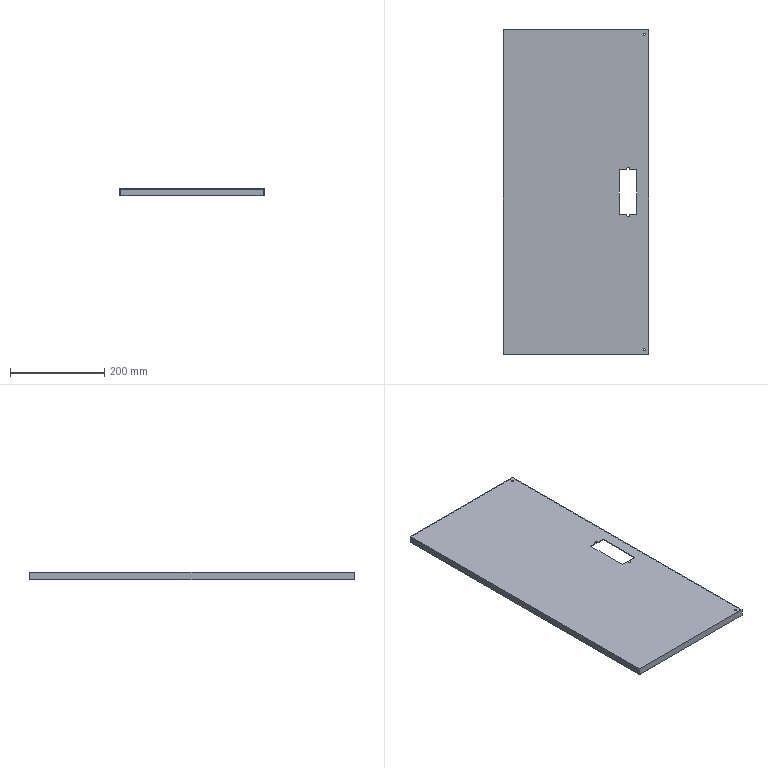Part | SolidWorks | features BaseBody 1 | 1 solid | 27 faces | box 308 x 688 x 15 mm | volume 352674 mm3 | plane 21 | cylinder 6 | commonest cylinder face diameters 4.5 x4 6 x2
STEP:
#1=CARTESIAN_POINT('',(-8.25,334.5,0.));
#2=VERTEX_POINT('',#1);
#3=CARTESIAN_POINT('',(-12.75,334.5,0.));
#4=VERTEX_POINT('',#3);
#5=CARTESIAN_POINT('',(-10.5,334.5,0.));
#6=DIRECTION('',(0.,0.,-1.));
#7=DIRECTION('',(-1.,0.,0.));
#8=AXIS2_PLACEMENT_3D('',#5,#6,#7);
#9=CIRCLE('',#8,2.25);
#10=EDGE_CURVE('',#2,#4,#9,.T.);
#11=ORIENTED_EDGE('',*,*,#10,.F.);
#12=CARTESIAN_POINT('',(-8.25,334.5,-1.5));
#13=VERTEX_POINT('',#12);
#14=CARTESIAN_POINT('',(-8.25,334.5,0.));
#15=DIRECTION('',(0.,0.,-1.));
#16=VECTOR('',#15,1000.);
#17=LINE('',#14,#16);
#18=EDGE_CURVE('',#2,#13,#17,.T.);
#19=ORIENTED_EDGE('',*,*,#18,.T.);
#20=CARTESIAN_POINT('',(-12.75,334.5,-1.5));
#21=VERTEX_POINT('',#20);
#22=CARTESIAN_POINT('',(-10.5,334.5,-1.5));
#23=DIRECTION('',(0.,0.,1.));
#24=DIRECTION('',(-1.,0.,0.));
#25=AXIS2_PLACEMENT_3D('',#22,#23,#24);
#26=CIRCLE('',#25,2.25);
#27=EDGE_CURVE('',#21,#13,#26,.T.);
#28=ORIENTED_EDGE('',*,*,#27,.F.);
#29=CARTESIAN_POINT('',(-12.75,334.5,0.));
#30=DIRECTION('',(0.,0.,-1.));
#31=VECTOR('',#30,1000.);
#32=LINE('',#29,#31);
#33=EDGE_CURVE('',#4,#21,#32,.T.);
#34=ORIENTED_EDGE('',*,*,#33,.F.);
#35=EDGE_LOOP('',(#11,#19,#28,#34));
#36=FACE_OUTER_BOUND('',#35,.T.);
#37=CARTESIAN_POINT('',(-10.5,334.5,0.));
#38=DIRECTION('',(0.,0.,-1.));
#39=DIRECTION('',(-1.,0.,0.));
#40=AXIS2_PLACEMENT_3D('',#37,#38,#39);
#41=CYLINDRICAL_SURFACE('',#40,2.25);
#42=ADVANCED_FACE('',(#36),#41,.F.);
#43=CARTESIAN_POINT('',(-8.25,-334.5,0.));
#44=VERTEX_POINT('',#43);
#45=CARTESIAN_POINT('',(-12.75,-334.5,0.));
#46=VERTEX_POINT('',#45);
#47=CARTESIAN_POINT('',(-10.5,-334.5,0.));
#48=DIRECTION('',(0.,0.,-1.));
#49=DIRECTION('',(-1.,0.,0.));
#50=AXIS2_PLACEMENT_3D('',#47,#48,#49);
#51=CIRCLE('',#50,2.25);
#52=EDGE_CURVE('',#44,#46,#51,.T.);
#53=ORIENTED_EDGE('',*,*,#52,.F.);
#54=CARTESIAN_POINT('',(-8.25,-334.5,-1.5));
#55=VERTEX_POINT('',#54);
#56=CARTESIAN_POINT('',(-8.25,-334.5,0.));
#57=DIRECTION('',(0.,0.,-1.));
#58=VECTOR('',#57,1000.);
#59=LINE('',#56,#58);
#60=EDGE_CURVE('',#44,#55,#59,.T.);
#61=ORIENTED_EDGE('',*,*,#60,.T.);
#62=CARTESIAN_POINT('',(-12.75,-334.5,-1.5));
#63=VERTEX_POINT('',#62);
#64=CARTESIAN_POINT('',(-10.5,-334.5,-1.5));
#65=DIRECTION('',(0.,0.,1.));
#66=DIRECTION('',(-1.,0.,0.));
#67=AXIS2_PLACEMENT_3D('',#64,#65,#66);
#68=CIRCLE('',#67,2.25);
#69=EDGE_CURVE('',#63,#55,#68,.T.);
#70=ORIENTED_EDGE('',*,*,#69,.F.);
#71=CARTESIAN_POINT('',(-12.75,-334.5,0.));
#72=DIRECTION('',(0.,0.,-1.));
#73=VECTOR('',#72,1000.);
#74=LINE('',#71,#73);
#75=EDGE_CURVE('',#46,#63,#74,.T.);
#76=ORIENTED_EDGE('',*,*,#75,.F.);
#77=EDGE_LOOP('',(#53,#61,#70,#76));
#78=FACE_OUTER_BOUND('',#77,.T.);
#79=CARTESIAN_POINT('',(-10.5,-334.5,0.));
#80=DIRECTION('',(0.,0.,-1.));
#81=DIRECTION('',(-1.,0.,0.));
#82=AXIS2_PLACEMENT_3D('',#79,#80,#81);
#83=CYLINDRICAL_SURFACE('',#82,2.25);
#84=ADVANCED_FACE('',(#78),#83,.F.);
#85=CARTESIAN_POINT('',(-1.,-344.,0.));
#86=VERTEX_POINT('',#85);
#87=CARTESIAN_POINT('',(-1.,344.,0.));
#88=VERTEX_POINT('',#87);
#89=CARTESIAN_POINT('',(-1.,0.,0.));
#90=DIRECTION('',(0.,1.,0.));
#91=VECTOR('',#90,1000.);
#92=LINE('',#89,#91);
#93=EDGE_CURVE('',#86,#88,#92,.T.);
#94=ORIENTED_EDGE('',*,*,#93,.T.);
#95=CARTESIAN_POINT('',(-309.,344.,0.));
#96=VERTEX_POINT('',#95);
#97=CARTESIAN_POINT('',(0.,344.,0.));
#98=DIRECTION('',(-1.,0.,0.));
#99=VECTOR('',#98,1000.);
#100=LINE('',#97,#99);
#101=EDGE_CURVE('',#88,#96,#100,.T.);
#102=ORIENTED_EDGE('',*,*,#101,.T.);
#103=CARTESIAN_POINT('',(-309.,-344.,0.));
#104=VERTEX_POINT('',#103);
#105=CARTESIAN_POINT('',(-309.,0.,0.));
#106=DIRECTION('',(0.,-1.,0.));
#107=VECTOR('',#106,1000.);
#108=LINE('',#105,#107);
#109=EDGE_CURVE('',#96,#104,#108,.T.);
#110=ORIENTED_EDGE('',*,*,#109,.T.);
#111=CARTESIAN_POINT('',(0.,-344.,0.));
#112=DIRECTION('',(1.,0.,0.));
#113=VECTOR('',#112,1000.);
#114=LINE('',#111,#113);
#115=EDGE_CURVE('',#104,#86,#114,.T.);
#116=ORIENTED_EDGE('',*,*,#115,.T.);
#117=EDGE_LOOP('',(#94,#102,#110,#116));
#118=FACE_OUTER_BOUND('',#117,.T.);
#119=CARTESIAN_POINT('',(-47.5,-49.5,0.));
#120=VERTEX_POINT('',#119);
#121=CARTESIAN_POINT('',(-47.5,-47.5,0.));
#122=VERTEX_POINT('',#121);
#123=CARTESIAN_POINT('',(-47.5,0.,0.));
#124=DIRECTION('',(0.,1.,0.));
#125=VECTOR('',#124,1000.);
#126=LINE('',#123,#125);
#127=EDGE_CURVE('',#120,#122,#126,.T.);
#128=ORIENTED_EDGE('',*,*,#127,.T.);
#129=CARTESIAN_POINT('',(-63.,-47.5,0.));
#130=VERTEX_POINT('',#129);
#131=CARTESIAN_POINT('',(0.,-47.5,0.));
#132=DIRECTION('',(-1.,0.,0.));
#133=VECTOR('',#132,1000.);
#134=LINE('',#131,#133);
#135=EDGE_CURVE('',#122,#130,#134,.T.);
#136=ORIENTED_EDGE('',*,*,#135,.T.);
#137=CARTESIAN_POINT('',(-63.,47.5,0.));
#138=VERTEX_POINT('',#137);
#139=CARTESIAN_POINT('',(-63.,0.,0.));
#140=DIRECTION('',(0.,1.,0.));
#141=VECTOR('',#140,1000.);
#142=LINE('',#139,#141);
#143=EDGE_CURVE('',#130,#138,#142,.T.);
#144=ORIENTED_EDGE('',*,*,#143,.T.);
#145=CARTESIAN_POINT('',(-47.5,47.5,0.));
#146=VERTEX_POINT('',#145);
#147=CARTESIAN_POINT('',(0.,47.5,0.));
#148=DIRECTION('',(1.,0.,0.));
#149=VECTOR('',#148,1000.);
#150=LINE('',#147,#149);
#151=EDGE_CURVE('',#138,#146,#150,.T.);
#152=ORIENTED_EDGE('',*,*,#151,.T.);
#153=CARTESIAN_POINT('',(-47.5,49.5,0.));
#154=VERTEX_POINT('',#153);
#155=CARTESIAN_POINT('',(-47.5,0.,0.));
#156=DIRECTION('',(0.,1.,0.));
#157=VECTOR('',#156,1000.);
#158=LINE('',#155,#157);
#159=EDGE_CURVE('',#146,#154,#158,.T.);
#160=ORIENTED_EDGE('',*,*,#159,.T.);
#161=CARTESIAN_POINT('',(-41.5,49.5,0.));
#162=VERTEX_POINT('',#161);
#163=CARTESIAN_POINT('',(-44.5,49.5,0.));
#164=DIRECTION('',(0.,0.,-1.));
#165=DIRECTION('',(1.,0.,0.));
#166=AXIS2_PLACEMENT_3D('',#163,#164,#165);
#167=CIRCLE('',#166,3.);
#168=EDGE_CURVE('',#154,#162,#167,.T.);
#169=ORIENTED_EDGE('',*,*,#168,.T.);
#170=CARTESIAN_POINT('',(-41.5,47.5,0.));
#171=VERTEX_POINT('',#170);
#172=CARTESIAN_POINT('',(-41.5,0.,0.));
#173=DIRECTION('',(0.,-1.,0.));
#174=VECTOR('',#173,1000.);
#175=LINE('',#172,#174);
#176=EDGE_CURVE('',#162,#171,#175,.T.);
#177=ORIENTED_EDGE('',*,*,#176,.T.);
#178=CARTESIAN_POINT('',(-26.,47.5,0.));
#179=VERTEX_POINT('',#178);
#180=CARTESIAN_POINT('',(0.,47.5,0.));
#181=DIRECTION('',(1.,0.,0.));
#182=VECTOR('',#181,1000.);
#183=LINE('',#180,#182);
#184=EDGE_CURVE('',#171,#179,#183,.T.);
#185=ORIENTED_EDGE('',*,*,#184,.T.);
#186=CARTESIAN_POINT('',(-26.,-47.5,0.));
#187=VERTEX_POINT('',#186);
#188=CARTESIAN_POINT('',(-26.,0.,0.));
#189=DIRECTION('',(0.,-1.,0.));
#190=VECTOR('',#189,1000.);
#191=LINE('',#188,#190);
#192=EDGE_CURVE('',#179,#187,#191,.T.);
#193=ORIENTED_EDGE('',*,*,#192,.T.);
#194=CARTESIAN_POINT('',(-41.5,-47.5,0.));
#195=VERTEX_POINT('',#194);
#196=CARTESIAN_POINT('',(0.,-47.5,0.));
#197=DIRECTION('',(-1.,0.,0.));
#198=VECTOR('',#197,1000.);
#199=LINE('',#196,#198);
#200=EDGE_CURVE('',#187,#195,#199,.T.);
#201=ORIENTED_EDGE('',*,*,#200,.T.);
#202=CARTESIAN_POINT('',(-41.5,-49.5,0.));
#203=VERTEX_POINT('',#202);
#204=CARTESIAN_POINT('',(-41.5,0.,0.));
#205=DIRECTION('',(0.,-1.,0.));
#206=VECTOR('',#205,1000.);
#207=LINE('',#204,#206);
#208=EDGE_CURVE('',#195,#203,#207,.T.);
#209=ORIENTED_EDGE('',*,*,#208,.T.);
#210=CARTESIAN_POINT('',(-44.5,-49.5,0.));
#211=DIRECTION('',(0.,0.,-1.));
#212=DIRECTION('',(1.,0.,0.));
#213=AXIS2_PLACEMENT_3D('',#210,#211,#212);
#214=CIRCLE('',#213,3.);
#215=EDGE_CURVE('',#203,#120,#214,.T.);
#216=ORIENTED_EDGE('',*,*,#215,.T.);
#217=EDGE_LOOP('',(#128,#136,#144,#152,#160,#169,#177,#185,#193,#201,#209,#216));
#218=FACE_BOUND('',#217,.T.);
#219=CARTESIAN_POINT('',(-10.5,334.5,0.));
#220=DIRECTION('',(0.,0.,-1.));
#221=DIRECTION('',(-1.,0.,0.));
#222=AXIS2_PLACEMENT_3D('',#219,#220,#221);
#223=CIRCLE('',#222,2.25);
#224=EDGE_CURVE('',#4,#2,#223,.T.);
#225=ORIENTED_EDGE('',*,*,#224,.T.);
#226=ORIENTED_EDGE('',*,*,#10,.T.);
#227=EDGE_LOOP('',(#225,#226));
#228=FACE_BOUND('',#227,.T.);
#229=CARTESIAN_POINT('',(-10.5,-334.5,0.));
#230=DIRECTION('',(0.,0.,-1.));
#231=DIRECTION('',(-1.,0.,0.));
#232=AXIS2_PLACEMENT_3D('',#229,#230,#231);
#233=CIRCLE('',#232,2.25);
#234=EDGE_CURVE('',#46,#44,#233,.T.);
#235=ORIENTED_EDGE('',*,*,#234,.T.);
#236=ORIENTED_EDGE('',*,*,#52,.T.);
#237=EDGE_LOOP('',(#235,#236));
#238=FACE_BOUND('',#237,.T.);
#239=CARTESIAN_POINT('',(0.,0.,0.));
#240=DIRECTION('',(0.,0.,1.));
#241=DIRECTION('',(1.,0.,0.));
#242=AXIS2_PLACEMENT_3D('',#239,#240,#241);
#243=PLANE('',#242);
#244=ADVANCED_FACE('',(#118,#218,#228,#238),#243,.T.);
#245=CARTESIAN_POINT('',(-1.,344.,-15.));
#246=VERTEX_POINT('',#245);
#247=CARTESIAN_POINT('',(-309.,344.,-15.));
#248=VERTEX_POINT('',#247);
#249=CARTESIAN_POINT('',(-309.,344.,-15.));
#250=DIRECTION('',(-1.,0.,0.));
#251=VECTOR('',#250,1000.);
#252=LINE('',#249,#251);
#253=EDGE_CURVE('',#246,#248,#252,.T.);
#254=ORIENTED_EDGE('',*,*,#253,.T.);
#255=CARTESIAN_POINT('',(-309.,344.,-15.));
#256=DIRECTION('',(0.,0.,1.));
#257=VECTOR('',#256,1000.);
#258=LINE('',#255,#257);
#259=EDGE_CURVE('',#248,#96,#258,.T.);
#260=ORIENTED_EDGE('',*,*,#259,.T.);
#261=ORIENTED_EDGE('',*,*,#101,.F.);
#262=CARTESIAN_POINT('',(-1.,344.,-15.));
#263=DIRECTION('',(0.,0.,-1.));
#264=VECTOR('',#263,1000.);
#265=LINE('',#262,#264);
#266=EDGE_CURVE('',#88,#246,#265,.T.);
#267=ORIENTED_EDGE('',*,*,#266,.T.);
#268=EDGE_LOOP('',(#254,#260,#261,#267));
#269=FACE_OUTER_BOUND('',#268,.T.);
#270=CARTESIAN_POINT('',(-309.,344.,-15.));
#271=DIRECTION('',(0.,1.,0.));
#272=DIRECTION('',(0.,0.,1.));
#273=AXIS2_PLACEMENT_3D('',#270,#271,#272);
#274=PLANE('',#273);
#275=ADVANCED_FACE('',(#269),#274,.T.);
#276=CARTESIAN_POINT('',(-1.,-344.,-15.));
#277=VERTEX_POINT('',#276);
#278=CARTESIAN_POINT('',(-1.,344.,-15.));
#279=DIRECTION('',(0.,1.,0.));
#280=VECTOR('',#279,1000.);
#281=LINE('',#278,#280);
#282=EDGE_CURVE('',#277,#246,#281,.T.);
#283=ORIENTED_EDGE('',*,*,#282,.T.);
#284=ORIENTED_EDGE('',*,*,#266,.F.);
#285=ORIENTED_EDGE('',*,*,#93,.F.);
#286=CARTESIAN_POINT('',(-1.,-344.,-15.));
#287=DIRECTION('',(0.,0.,-1.));
#288=VECTOR('',#287,1000.);
#289=LINE('',#286,#288);
#290=EDGE_CURVE('',#86,#277,#289,.T.);
#291=ORIENTED_EDGE('',*,*,#290,.T.);
#292=EDGE_LOOP('',(#283,#284,#285,#291));
#293=FACE_OUTER_BOUND('',#292,.T.);
#294=CARTESIAN_POINT('',(-1.,344.,-15.));
#295=DIRECTION('',(1.,0.,0.));
#296=DIRECTION('',(0.,1.,0.));
#297=AXIS2_PLACEMENT_3D('',#294,#295,#296);
#298=PLANE('',#297);
#299=ADVANCED_FACE('',(#293),#298,.T.);
#300=CARTESIAN_POINT('',(-309.,-344.,-15.));
#301=VERTEX_POINT('',#300);
#302=CARTESIAN_POINT('',(-309.,-344.,-15.));
#303=DIRECTION('',(1.,0.,0.));
#304=VECTOR('',#303,1000.);
#305=LINE('',#302,#304);
#306=EDGE_CURVE('',#301,#277,#305,.T.);
#307=ORIENTED_EDGE('',*,*,#306,.T.);
#308=ORIENTED_EDGE('',*,*,#290,.F.);
#309=ORIENTED_EDGE('',*,*,#115,.F.);
#310=CARTESIAN_POINT('',(-309.,-344.,-15.));
#311=DIRECTION('',(0.,0.,-1.));
#312=VECTOR('',#311,1000.);
#313=LINE('',#310,#312);
#314=EDGE_CURVE('',#104,#301,#313,.T.);
#315=ORIENTED_EDGE('',*,*,#314,.T.);
#316=EDGE_LOOP('',(#307,#308,#309,#315));
#317=FACE_OUTER_BOUND('',#316,.T.);
#318=CARTESIAN_POINT('',(-309.,-344.,-15.));
#319=DIRECTION('',(0.,-1.,0.));
#320=DIRECTION('',(1.,0.,0.));
#321=AXIS2_PLACEMENT_3D('',#318,#319,#320);
#322=PLANE('',#321);
#323=ADVANCED_FACE('',(#317),#322,.T.);
#324=CARTESIAN_POINT('',(-309.,344.,-15.));
#325=DIRECTION('',(0.,-1.,0.));
#326=VECTOR('',#325,1000.);
#327=LINE('',#324,#326);
#328=EDGE_CURVE('',#248,#301,#327,.T.);
#329=ORIENTED_EDGE('',*,*,#328,.T.);
#330=ORIENTED_EDGE('',*,*,#314,.F.);
#331=ORIENTED_EDGE('',*,*,#109,.F.);
#332=ORIENTED_EDGE('',*,*,#259,.F.);
#333=EDGE_LOOP('',(#329,#330,#331,#332));
#334=FACE_OUTER_BOUND('',#333,.T.);
#335=CARTESIAN_POINT('',(-309.,344.,-15.));
#336=DIRECTION('',(-1.,0.,0.));
#337=DIRECTION('',(0.,-1.,0.));
#338=AXIS2_PLACEMENT_3D('',#335,#336,#337);
#339=PLANE('',#338);
#340=ADVANCED_FACE('',(#334),#339,.T.);
#341=ORIENTED_EDGE('',*,*,#135,.F.);
#342=CARTESIAN_POINT('',(-47.5,-47.5,-1.5));
#343=VERTEX_POINT('',#342);
#344=CARTESIAN_POINT('',(-47.5,-47.5,-15.));
#345=DIRECTION('',(0.,0.,1.));
#346=VECTOR('',#345,1000.);
#347=LINE('',#344,#346);
#348=EDGE_CURVE('',#343,#122,#347,.T.);
#349=ORIENTED_EDGE('',*,*,#348,.F.);
#350=CARTESIAN_POINT('',(-63.,-47.5,-1.5));
#351=VERTEX_POINT('',#350);
#352=CARTESIAN_POINT('',(-63.,-47.5,-1.5));
#353=DIRECTION('',(1.,0.,0.));
#354=VECTOR('',#353,1000.);
#355=LINE('',#352,#354);
#356=EDGE_CURVE('',#351,#343,#355,.T.);
#357=ORIENTED_EDGE('',*,*,#356,.F.);
#358=CARTESIAN_POINT('',(-63.,-47.5,-15.));
#359=DIRECTION('',(0.,0.,-1.));
#360=VECTOR('',#359,1000.);
#361=LINE('',#358,#360);
#362=EDGE_CURVE('',#130,#351,#361,.T.);
#363=ORIENTED_EDGE('',*,*,#362,.F.);
#364=EDGE_LOOP('',(#341,#349,#357,#363));
#365=FACE_OUTER_BOUND('',#364,.T.);
#366=CARTESIAN_POINT('',(-63.,-47.5,-15.));
#367=DIRECTION('',(0.,-1.,0.));
#368=DIRECTION('',(1.,0.,0.));
#369=AXIS2_PLACEMENT_3D('',#366,#367,#368);
#370=PLANE('',#369);
#371=ADVANCED_FACE('',(#365),#370,.F.);
#372=ORIENTED_EDGE('',*,*,#127,.F.);
#373=CARTESIAN_POINT('',(-47.5,-49.5,-1.5));
#374=VERTEX_POINT('',#373);
#375=CARTESIAN_POINT('',(-47.5,-49.5,-15.));
#376=DIRECTION('',(0.,0.,1.));
#377=VECTOR('',#376,1000.);
#378=LINE('',#375,#377);
#379=EDGE_CURVE('',#374,#120,#378,.T.);
#380=ORIENTED_EDGE('',*,*,#379,.F.);
#381=CARTESIAN_POINT('',(-47.5,-49.5,-1.5));
#382=DIRECTION('',(0.,-1.,0.));
#383=VECTOR('',#382,1000.);
#384=LINE('',#381,#383);
#385=EDGE_CURVE('',#343,#374,#384,.T.);
#386=ORIENTED_EDGE('',*,*,#385,.F.);
#387=ORIENTED_EDGE('',*,*,#348,.T.);
#388=EDGE_LOOP('',(#372,#380,#386,#387));
#389=FACE_OUTER_BOUND('',#388,.T.);
#390=CARTESIAN_POINT('',(-47.5,-49.5,-15.));
#391=DIRECTION('',(-1.,0.,0.));
#392=DIRECTION('',(0.,-1.,0.));
#393=AXIS2_PLACEMENT_3D('',#390,#391,#392);
#394=PLANE('',#393);
#395=ADVANCED_FACE('',(#389),#394,.F.);
#396=ORIENTED_EDGE('',*,*,#215,.F.);
#397=CARTESIAN_POINT('',(-41.5,-49.5,-1.5));
#398=VERTEX_POINT('',#397);
#399=CARTESIAN_POINT('',(-41.5,-49.5,-15.));
#400=DIRECTION('',(0.,0.,1.));
#401=VECTOR('',#400,1000.);
#402=LINE('',#399,#401);
#403=EDGE_CURVE('',#398,#203,#402,.T.);
#404=ORIENTED_EDGE('',*,*,#403,.F.);
#405=CARTESIAN_POINT('',(-44.5,-49.5,-1.5));
#406=DIRECTION('',(0.,0.,1.));
#407=DIRECTION('',(1.,0.,0.));
#408=AXIS2_PLACEMENT_3D('',#405,#406,#407);
#409=CIRCLE('',#408,3.);
#410=EDGE_CURVE('',#374,#398,#409,.T.);
#411=ORIENTED_EDGE('',*,*,#410,.F.);
#412=ORIENTED_EDGE('',*,*,#379,.T.);
#413=EDGE_LOOP('',(#396,#404,#411,#412));
#414=FACE_OUTER_BOUND('',#413,.T.);
#415=CARTESIAN_POINT('',(-44.5,-49.5,-15.));
#416=DIRECTION('',(0.,0.,1.));
#417=DIRECTION('',(1.,0.,0.));
#418=AXIS2_PLACEMENT_3D('',#415,#416,#417);
#419=CYLINDRICAL_SURFACE('',#418,3.);
#420=ADVANCED_FACE('',(#414),#419,.F.);
#421=ORIENTED_EDGE('',*,*,#208,.F.);
#422=CARTESIAN_POINT('',(-41.5,-47.5,-1.5));
#423=VERTEX_POINT('',#422);
#424=CARTESIAN_POINT('',(-41.5,-47.5,-15.));
#425=DIRECTION('',(0.,0.,1.));
#426=VECTOR('',#425,1000.);
#427=LINE('',#424,#426);
#428=EDGE_CURVE('',#423,#195,#427,.T.);
#429=ORIENTED_EDGE('',*,*,#428,.F.);
#430=CARTESIAN_POINT('',(-41.5,-49.5,-1.5));
#431=DIRECTION('',(0.,1.,0.));
#432=VECTOR('',#431,1000.);
#433=LINE('',#430,#432);
#434=EDGE_CURVE('',#398,#423,#433,.T.);
#435=ORIENTED_EDGE('',*,*,#434,.F.);
#436=ORIENTED_EDGE('',*,*,#403,.T.);
#437=EDGE_LOOP('',(#421,#429,#435,#436));
#438=FACE_OUTER_BOUND('',#437,.T.);
#439=CARTESIAN_POINT('',(-41.5,-49.5,-15.));
#440=DIRECTION('',(1.,0.,0.));
#441=DIRECTION('',(0.,1.,0.));
#442=AXIS2_PLACEMENT_3D('',#439,#440,#441);
#443=PLANE('',#442);
#444=ADVANCED_FACE('',(#438),#443,.F.);
#445=ORIENTED_EDGE('',*,*,#200,.F.);
#446=CARTESIAN_POINT('',(-26.,-47.5,-1.5));
#447=VERTEX_POINT('',#446);
#448=CARTESIAN_POINT('',(-26.,-47.5,-15.));
#449=DIRECTION('',(0.,0.,1.));
#450=VECTOR('',#449,1000.);
#451=LINE('',#448,#450);
#452=EDGE_CURVE('',#447,#187,#451,.T.);
#453=ORIENTED_EDGE('',*,*,#452,.F.);
#454=CARTESIAN_POINT('',(-41.5,-47.5,-1.5));
#455=DIRECTION('',(1.,0.,0.));
#456=VECTOR('',#455,1000.);
#457=LINE('',#454,#456);
#458=EDGE_CURVE('',#423,#447,#457,.T.);
#459=ORIENTED_EDGE('',*,*,#458,.F.);
#460=ORIENTED_EDGE('',*,*,#428,.T.);
#461=EDGE_LOOP('',(#445,#453,#459,#460));
#462=FACE_OUTER_BOUND('',#461,.T.);
#463=CARTESIAN_POINT('',(-41.5,-47.5,-15.));
#464=DIRECTION('',(0.,-1.,0.));
#465=DIRECTION('',(1.,0.,0.));
#466=AXIS2_PLACEMENT_3D('',#463,#464,#465);
#467=PLANE('',#466);
#468=ADVANCED_FACE('',(#462),#467,.F.);
#469=ORIENTED_EDGE('',*,*,#192,.F.);
#470=CARTESIAN_POINT('',(-26.,47.5,-1.5));
#471=VERTEX_POINT('',#470);
#472=CARTESIAN_POINT('',(-26.,47.5,-15.));
#473=DIRECTION('',(0.,0.,1.));
#474=VECTOR('',#473,1000.);
#475=LINE('',#472,#474);
#476=EDGE_CURVE('',#471,#179,#475,.T.);
#477=ORIENTED_EDGE('',*,*,#476,.F.);
#478=CARTESIAN_POINT('',(-26.,47.5,-1.5));
#479=DIRECTION('',(0.,1.,0.));
#480=VECTOR('',#479,1000.);
#481=LINE('',#478,#480);
#482=EDGE_CURVE('',#447,#471,#481,.T.);
#483=ORIENTED_EDGE('',*,*,#482,.F.);
#484=ORIENTED_EDGE('',*,*,#452,.T.);
#485=EDGE_LOOP('',(#469,#477,#483,#484));
#486=FACE_OUTER_BOUND('',#485,.T.);
#487=CARTESIAN_POINT('',(-26.,47.5,-15.));
#488=DIRECTION('',(1.,0.,0.));
#489=DIRECTION('',(0.,1.,0.));
#490=AXIS2_PLACEMENT_3D('',#487,#488,#489);
#491=PLANE('',#490);
#492=ADVANCED_FACE('',(#486),#491,.F.);
#493=ORIENTED_EDGE('',*,*,#184,.F.);
#494=CARTESIAN_POINT('',(-41.5,47.5,-1.5));
#495=VERTEX_POINT('',#494);
#496=CARTESIAN_POINT('',(-41.5,47.5,-15.));
#497=DIRECTION('',(0.,0.,1.));
#498=VECTOR('',#497,1000.);
#499=LINE('',#496,#498);
#500=EDGE_CURVE('',#495,#171,#499,.T.);
#501=ORIENTED_EDGE('',*,*,#500,.F.);
#502=CARTESIAN_POINT('',(-41.5,47.5,-1.5));
#503=DIRECTION('',(-1.,0.,0.));
#504=VECTOR('',#503,1000.);
#505=LINE('',#502,#504);
#506=EDGE_CURVE('',#471,#495,#505,.T.);
#507=ORIENTED_EDGE('',*,*,#506,.F.);
#508=ORIENTED_EDGE('',*,*,#476,.T.);
#509=EDGE_LOOP('',(#493,#501,#507,#508));
#510=FACE_OUTER_BOUND('',#509,.T.);
#511=CARTESIAN_POINT('',(-41.5,47.5,-15.));
#512=DIRECTION('',(0.,1.,0.));
#513=DIRECTION('',(0.,0.,1.));
#514=AXIS2_PLACEMENT_3D('',#511,#512,#513);
#515=PLANE('',#514);
#516=ADVANCED_FACE('',(#510),#515,.F.);
#517=ORIENTED_EDGE('',*,*,#176,.F.);
#518=CARTESIAN_POINT('',(-41.5,49.5,-1.5));
#519=VERTEX_POINT('',#518);
#520=CARTESIAN_POINT('',(-41.5,49.5,-15.));
#521=DIRECTION('',(0.,0.,1.));
#522=VECTOR('',#521,1000.);
#523=LINE('',#520,#522);
#524=EDGE_CURVE('',#519,#162,#523,.T.);
#525=ORIENTED_EDGE('',*,*,#524,.F.);
#526=CARTESIAN_POINT('',(-41.5,49.5,-1.5));
#527=DIRECTION('',(0.,1.,0.));
#528=VECTOR('',#527,1000.);
#529=LINE('',#526,#528);
#530=EDGE_CURVE('',#495,#519,#529,.T.);
#531=ORIENTED_EDGE('',*,*,#530,.F.);
#532=ORIENTED_EDGE('',*,*,#500,.T.);
#533=EDGE_LOOP('',(#517,#525,#531,#532));
#534=FACE_OUTER_BOUND('',#533,.T.);
#535=CARTESIAN_POINT('',(-41.5,49.5,-15.));
#536=DIRECTION('',(1.,0.,0.));
#537=DIRECTION('',(0.,1.,0.));
#538=AXIS2_PLACEMENT_3D('',#535,#536,#537);
#539=PLANE('',#538);
#540=ADVANCED_FACE('',(#534),#539,.F.);
#541=ORIENTED_EDGE('',*,*,#168,.F.);
#542=CARTESIAN_POINT('',(-47.5,49.5,-1.5));
#543=VERTEX_POINT('',#542);
#544=CARTESIAN_POINT('',(-47.5,49.5,-15.));
#545=DIRECTION('',(0.,0.,1.));
#546=VECTOR('',#545,1000.);
#547=LINE('',#544,#546);
#548=EDGE_CURVE('',#543,#154,#547,.T.);
#549=ORIENTED_EDGE('',*,*,#548,.F.);
#550=CARTESIAN_POINT('',(-44.5,49.5,-1.5));
#551=DIRECTION('',(0.,0.,1.));
#552=DIRECTION('',(1.,0.,0.));
#553=AXIS2_PLACEMENT_3D('',#550,#551,#552);
#554=CIRCLE('',#553,3.);
#555=EDGE_CURVE('',#519,#543,#554,.T.);
#556=ORIENTED_EDGE('',*,*,#555,.F.);
#557=ORIENTED_EDGE('',*,*,#524,.T.);
#558=EDGE_LOOP('',(#541,#549,#556,#557));
#559=FACE_OUTER_BOUND('',#558,.T.);
#560=CARTESIAN_POINT('',(-44.5,49.5,-15.));
#561=DIRECTION('',(0.,0.,1.));
#562=DIRECTION('',(1.,0.,0.));
#563=AXIS2_PLACEMENT_3D('',#560,#561,#562);
#564=CYLINDRICAL_SURFACE('',#563,3.);
#565=ADVANCED_FACE('',(#559),#564,.F.);
#566=ORIENTED_EDGE('',*,*,#159,.F.);
#567=CARTESIAN_POINT('',(-47.5,47.5,-1.5));
#568=VERTEX_POINT('',#567);
#569=CARTESIAN_POINT('',(-47.5,47.5,-15.));
#570=DIRECTION('',(0.,0.,1.));
#571=VECTOR('',#570,1000.);
#572=LINE('',#569,#571);
#573=EDGE_CURVE('',#568,#146,#572,.T.);
#574=ORIENTED_EDGE('',*,*,#573,.F.);
#575=CARTESIAN_POINT('',(-47.5,49.5,-1.5));
#576=DIRECTION('',(0.,-1.,0.));
#577=VECTOR('',#576,1000.);
#578=LINE('',#575,#577);
#579=EDGE_CURVE('',#543,#568,#578,.T.);
#580=ORIENTED_EDGE('',*,*,#579,.F.);
#581=ORIENTED_EDGE('',*,*,#548,.T.);
#582=EDGE_LOOP('',(#566,#574,#580,#581));
#583=FACE_OUTER_BOUND('',#582,.T.);
#584=CARTESIAN_POINT('',(-47.5,49.5,-15.));
#585=DIRECTION('',(-1.,0.,0.));
#586=DIRECTION('',(0.,0.,1.));
#587=AXIS2_PLACEMENT_3D('',#584,#585,#586);
#588=PLANE('',#587);
#589=ADVANCED_FACE('',(#583),#588,.F.);
#590=ORIENTED_EDGE('',*,*,#151,.F.);
#591=CARTESIAN_POINT('',(-63.,47.5,-1.5));
#592=VERTEX_POINT('',#591);
#593=CARTESIAN_POINT('',(-63.,47.5,-15.));
#594=DIRECTION('',(0.,0.,1.));
#595=VECTOR('',#594,1000.);
#596=LINE('',#593,#595);
#597=EDGE_CURVE('',#592,#138,#596,.T.);
#598=ORIENTED_EDGE('',*,*,#597,.F.);
#599=CARTESIAN_POINT('',(-63.,47.5,-1.5));
#600=DIRECTION('',(-1.,0.,0.));
#601=VECTOR('',#600,1000.);
#602=LINE('',#599,#601);
#603=EDGE_CURVE('',#568,#592,#602,.T.);
#604=ORIENTED_EDGE('',*,*,#603,.F.);
#605=ORIENTED_EDGE('',*,*,#573,.T.);
#606=EDGE_LOOP('',(#590,#598,#604,#605));
#607=FACE_OUTER_BOUND('',#606,.T.);
#608=CARTESIAN_POINT('',(-63.,47.5,-15.));
#609=DIRECTION('',(0.,1.,0.));
#610=DIRECTION('',(0.,0.,1.));
#611=AXIS2_PLACEMENT_3D('',#608,#609,#610);
#612=PLANE('',#611);
#613=ADVANCED_FACE('',(#607),#612,.F.);
#614=ORIENTED_EDGE('',*,*,#143,.F.);
#615=ORIENTED_EDGE('',*,*,#362,.T.);
#616=CARTESIAN_POINT('',(-63.,47.5,-1.5));
#617=DIRECTION('',(0.,-1.,0.));
#618=VECTOR('',#617,1000.);
#619=LINE('',#616,#618);
#620=EDGE_CURVE('',#592,#351,#619,.T.);
#621=ORIENTED_EDGE('',*,*,#620,.F.);
#622=ORIENTED_EDGE('',*,*,#597,.T.);
#623=EDGE_LOOP('',(#614,#615,#621,#622));
#624=FACE_OUTER_BOUND('',#623,.T.);
#625=CARTESIAN_POINT('',(-63.,47.5,-15.));
#626=DIRECTION('',(-1.,0.,0.));
#627=DIRECTION('',(0.,-1.,0.));
#628=AXIS2_PLACEMENT_3D('',#625,#626,#627);
#629=PLANE('',#628);
#630=ADVANCED_FACE('',(#624),#629,.F.);
#631=ORIENTED_EDGE('',*,*,#18,.F.);
#632=ORIENTED_EDGE('',*,*,#224,.F.);
#633=ORIENTED_EDGE('',*,*,#33,.T.);
#634=CARTESIAN_POINT('',(-10.5,334.5,-1.5));
#635=DIRECTION('',(0.,0.,1.));
#636=DIRECTION('',(-1.,0.,0.));
#637=AXIS2_PLACEMENT_3D('',#634,#635,#636);
#638=CIRCLE('',#637,2.25);
#639=EDGE_CURVE('',#13,#21,#638,.T.);
#640=ORIENTED_EDGE('',*,*,#639,.F.);
#641=EDGE_LOOP('',(#631,#632,#633,#640));
#642=FACE_OUTER_BOUND('',#641,.T.);
#643=CARTESIAN_POINT('',(-10.5,334.5,0.));
#644=DIRECTION('',(0.,0.,-1.));
#645=DIRECTION('',(-1.,0.,0.));
#646=AXIS2_PLACEMENT_3D('',#643,#644,#645);
#647=CYLINDRICAL_SURFACE('',#646,2.25);
#648=ADVANCED_FACE('',(#642),#647,.F.);
#649=ORIENTED_EDGE('',*,*,#60,.F.);
#650=ORIENTED_EDGE('',*,*,#234,.F.);
#651=ORIENTED_EDGE('',*,*,#75,.T.);
#652=CARTESIAN_POINT('',(-10.5,-334.5,-1.5));
#653=DIRECTION('',(0.,0.,1.));
#654=DIRECTION('',(-1.,0.,0.));
#655=AXIS2_PLACEMENT_3D('',#652,#653,#654);
#656=CIRCLE('',#655,2.25);
#657=EDGE_CURVE('',#55,#63,#656,.T.);
#658=ORIENTED_EDGE('',*,*,#657,.F.);
#659=EDGE_LOOP('',(#649,#650,#651,#658));
#660=FACE_OUTER_BOUND('',#659,.T.);
#661=CARTESIAN_POINT('',(-10.5,-334.5,0.));
#662=DIRECTION('',(0.,0.,-1.));
#663=DIRECTION('',(-1.,0.,0.));
#664=AXIS2_PLACEMENT_3D('',#661,#662,#663);
#665=CYLINDRICAL_SURFACE('',#664,2.25);
#666=ADVANCED_FACE('',(#660),#665,.F.);
#667=ORIENTED_EDGE('',*,*,#253,.F.);
#668=ORIENTED_EDGE('',*,*,#282,.F.);
#669=ORIENTED_EDGE('',*,*,#306,.F.);
#670=ORIENTED_EDGE('',*,*,#328,.F.);
#671=EDGE_LOOP('',(#667,#668,#669,#670));
#672=FACE_OUTER_BOUND('',#671,.T.);
#673=CARTESIAN_POINT('',(-307.5,-342.5,-15.));
#674=VERTEX_POINT('',#673);
#675=CARTESIAN_POINT('',(-307.5,342.5,-15.));
#676=VERTEX_POINT('',#675);
#677=CARTESIAN_POINT('',(-307.5,0.,-15.));
#678=DIRECTION('',(0.,1.,0.));
#679=VECTOR('',#678,1000.);
#680=LINE('',#677,#679);
#681=EDGE_CURVE('',#674,#676,#680,.T.);
#682=ORIENTED_EDGE('',*,*,#681,.F.);
#683=CARTESIAN_POINT('',(-2.5,-342.5,-15.));
#684=VERTEX_POINT('',#683);
#685=CARTESIAN_POINT('',(0.,-342.5,-15.));
#686=DIRECTION('',(-1.,0.,0.));
#687=VECTOR('',#686,1000.);
#688=LINE('',#685,#687);
#689=EDGE_CURVE('',#684,#674,#688,.T.);
#690=ORIENTED_EDGE('',*,*,#689,.F.);
#691=CARTESIAN_POINT('',(-2.5,342.5,-15.));
#692=VERTEX_POINT('',#691);
#693=CARTESIAN_POINT('',(-2.5,0.,-15.));
#694=DIRECTION('',(0.,-1.,0.));
#695=VECTOR('',#694,1000.);
#696=LINE('',#693,#695);
#697=EDGE_CURVE('',#692,#684,#696,.T.);
#698=ORIENTED_EDGE('',*,*,#697,.F.);
#699=CARTESIAN_POINT('',(0.,342.5,-15.));
#700=DIRECTION('',(1.,0.,0.));
#701=VECTOR('',#700,1000.);
#702=LINE('',#699,#701);
#703=EDGE_CURVE('',#676,#692,#702,.T.);
#704=ORIENTED_EDGE('',*,*,#703,.F.);
#705=EDGE_LOOP('',(#682,#690,#698,#704));
#706=FACE_BOUND('',#705,.T.);
#707=CARTESIAN_POINT('',(0.,0.,-15.));
#708=DIRECTION('',(0.,0.,1.));
#709=DIRECTION('',(1.,0.,0.));
#710=AXIS2_PLACEMENT_3D('',#707,#708,#709);
#711=PLANE('',#710);
#712=ADVANCED_FACE('',(#672,#706),#711,.F.);
#713=CARTESIAN_POINT('',(-2.5,342.5,-1.5));
#714=VERTEX_POINT('',#713);
#715=CARTESIAN_POINT('',(-307.5,342.5,-1.5));
#716=VERTEX_POINT('',#715);
#717=CARTESIAN_POINT('',(0.,342.5,-1.5));
#718=DIRECTION('',(-1.,0.,0.));
#719=VECTOR('',#718,1000.);
#720=LINE('',#717,#719);
#721=EDGE_CURVE('',#714,#716,#720,.T.);
#722=ORIENTED_EDGE('',*,*,#721,.F.);
#723=CARTESIAN_POINT('',(-2.5,-342.5,-1.5));
#724=VERTEX_POINT('',#723);
#725=CARTESIAN_POINT('',(-2.5,0.,-1.5));
#726=DIRECTION('',(0.,1.,0.));
#727=VECTOR('',#726,1000.);
#728=LINE('',#725,#727);
#729=EDGE_CURVE('',#724,#714,#728,.T.);
#730=ORIENTED_EDGE('',*,*,#729,.F.);
#731=CARTESIAN_POINT('',(-307.5,-342.5,-1.5));
#732=VERTEX_POINT('',#731);
#733=CARTESIAN_POINT('',(0.,-342.5,-1.5));
#734=DIRECTION('',(1.,0.,0.));
#735=VECTOR('',#734,1000.);
#736=LINE('',#733,#735);
#737=EDGE_CURVE('',#732,#724,#736,.T.);
#738=ORIENTED_EDGE('',*,*,#737,.F.);
#739=CARTESIAN_POINT('',(-307.5,0.,-1.5));
#740=DIRECTION('',(0.,-1.,0.));
#741=VECTOR('',#740,1000.);
#742=LINE('',#739,#741);
#743=EDGE_CURVE('',#716,#732,#742,.T.);
#744=ORIENTED_EDGE('',*,*,#743,.F.);
#745=EDGE_LOOP('',(#722,#730,#738,#744));
#746=FACE_OUTER_BOUND('',#745,.T.);
#747=ORIENTED_EDGE('',*,*,#620,.T.);
#748=ORIENTED_EDGE('',*,*,#356,.T.);
#749=ORIENTED_EDGE('',*,*,#385,.T.);
#750=ORIENTED_EDGE('',*,*,#410,.T.);
#751=ORIENTED_EDGE('',*,*,#434,.T.);
#752=ORIENTED_EDGE('',*,*,#458,.T.);
#753=ORIENTED_EDGE('',*,*,#482,.T.);
#754=ORIENTED_EDGE('',*,*,#506,.T.);
#755=ORIENTED_EDGE('',*,*,#530,.T.);
#756=ORIENTED_EDGE('',*,*,#555,.T.);
#757=ORIENTED_EDGE('',*,*,#579,.T.);
#758=ORIENTED_EDGE('',*,*,#603,.T.);
#759=EDGE_LOOP('',(#747,#748,#749,#750,#751,#752,#753,#754,#755,#756,#757,#758));
#760=FACE_BOUND('',#759,.T.);
#761=ORIENTED_EDGE('',*,*,#27,.T.);
#762=ORIENTED_EDGE('',*,*,#639,.T.);
#763=EDGE_LOOP('',(#761,#762));
#764=FACE_BOUND('',#763,.T.);
#765=ORIENTED_EDGE('',*,*,#69,.T.);
#766=ORIENTED_EDGE('',*,*,#657,.T.);
#767=EDGE_LOOP('',(#765,#766));
#768=FACE_BOUND('',#767,.T.);
#769=CARTESIAN_POINT('',(0.,0.,-1.5));
#770=DIRECTION('',(0.,0.,1.));
#771=DIRECTION('',(1.,0.,0.));
#772=AXIS2_PLACEMENT_3D('',#769,#770,#771);
#773=PLANE('',#772);
#774=ADVANCED_FACE('',(#746,#760,#764,#768),#773,.F.);
#775=CARTESIAN_POINT('',(-307.5,342.5,-15.));
#776=DIRECTION('',(0.,0.,1.));
#777=VECTOR('',#776,1000.);
#778=LINE('',#775,#777);
#779=EDGE_CURVE('',#676,#716,#778,.T.);
#780=ORIENTED_EDGE('',*,*,#779,.F.);
#781=ORIENTED_EDGE('',*,*,#703,.T.);
#782=CARTESIAN_POINT('',(-2.5,342.5,-15.));
#783=DIRECTION('',(0.,0.,-1.));
#784=VECTOR('',#783,1000.);
#785=LINE('',#782,#784);
#786=EDGE_CURVE('',#714,#692,#785,.T.);
#787=ORIENTED_EDGE('',*,*,#786,.F.);
#788=ORIENTED_EDGE('',*,*,#721,.T.);
#789=EDGE_LOOP('',(#780,#781,#787,#788));
#790=FACE_OUTER_BOUND('',#789,.T.);
#791=CARTESIAN_POINT('',(-309.,342.5,-15.));
#792=DIRECTION('',(0.,1.,0.));
#793=DIRECTION('',(0.,0.,1.));
#794=AXIS2_PLACEMENT_3D('',#791,#792,#793);
#795=PLANE('',#794);
#796=ADVANCED_FACE('',(#790),#795,.F.);
#797=CARTESIAN_POINT('',(-307.5,-342.5,-15.));
#798=DIRECTION('',(0.,0.,1.));
#799=VECTOR('',#798,1000.);
#800=LINE('',#797,#799);
#801=EDGE_CURVE('',#674,#732,#800,.T.);
#802=ORIENTED_EDGE('',*,*,#801,.F.);
#803=ORIENTED_EDGE('',*,*,#681,.T.);
#804=ORIENTED_EDGE('',*,*,#779,.T.);
#805=ORIENTED_EDGE('',*,*,#743,.T.);
#806=EDGE_LOOP('',(#802,#803,#804,#805));
#807=FACE_OUTER_BOUND('',#806,.T.);
#808=CARTESIAN_POINT('',(-307.5,344.,-15.));
#809=DIRECTION('',(-1.,0.,0.));
#810=DIRECTION('',(0.,-1.,0.));
#811=AXIS2_PLACEMENT_3D('',#808,#809,#810);
#812=PLANE('',#811);
#813=ADVANCED_FACE('',(#807),#812,.F.);
#814=CARTESIAN_POINT('',(-2.5,-342.5,-15.));
#815=DIRECTION('',(0.,0.,1.));
#816=VECTOR('',#815,1000.);
#817=LINE('',#814,#816);
#818=EDGE_CURVE('',#684,#724,#817,.T.);
#819=ORIENTED_EDGE('',*,*,#818,.F.);
#820=ORIENTED_EDGE('',*,*,#689,.T.);
#821=ORIENTED_EDGE('',*,*,#801,.T.);
#822=ORIENTED_EDGE('',*,*,#737,.T.);
#823=EDGE_LOOP('',(#819,#820,#821,#822));
#824=FACE_OUTER_BOUND('',#823,.T.);
#825=CARTESIAN_POINT('',(-309.,-342.5,-15.));
#826=DIRECTION('',(0.,-1.,0.));
#827=DIRECTION('',(1.,0.,0.));
#828=AXIS2_PLACEMENT_3D('',#825,#826,#827);
#829=PLANE('',#828);
#830=ADVANCED_FACE('',(#824),#829,.F.);
#831=ORIENTED_EDGE('',*,*,#786,.T.);
#832=ORIENTED_EDGE('',*,*,#697,.T.);
#833=ORIENTED_EDGE('',*,*,#818,.T.);
#834=ORIENTED_EDGE('',*,*,#729,.T.);
#835=EDGE_LOOP('',(#831,#832,#833,#834));
#836=FACE_OUTER_BOUND('',#835,.T.);
#837=CARTESIAN_POINT('',(-2.5,344.,-15.));
#838=DIRECTION('',(1.,0.,0.));
#839=DIRECTION('',(0.,1.,0.));
#840=AXIS2_PLACEMENT_3D('',#837,#838,#839);
#841=PLANE('',#840);
#842=ADVANCED_FACE('',(#836),#841,.F.);
#843=CLOSED_SHELL('',(#42,#84,#244,#275,#299,#323,#340,#371,#395,#420,#444,#468,#492,#516,#540,#565,#589,#613,#630,#648,#666,#712,#774,#796,#813,#830,#842));
#844=MANIFOLD_SOLID_BREP('',#843);
#845=CARTESIAN_POINT('',(0.,0.,0.));
#846=DIRECTION('',(0.,0.,1.));
#847=DIRECTION('',(1.,0.,0.));
#848=AXIS2_PLACEMENT_3D('',#845,#846,#847);
#849=(LENGTH_UNIT()NAMED_UNIT(*)SI_UNIT(.MILLI.,.METRE.));
#850=UNCERTAINTY_MEASURE_WITH_UNIT(LENGTH_MEASURE(0.00001),#849,'','');
#851=(NAMED_UNIT(*)PLANE_ANGLE_UNIT()SI_UNIT($,.RADIAN.));
#852=(NAMED_UNIT(*)SI_UNIT($,.STERADIAN.)SOLID_ANGLE_UNIT());
#853=(GEOMETRIC_REPRESENTATION_CONTEXT(3)GLOBAL_UNCERTAINTY_ASSIGNED_CONTEXT((#850))GLOBAL_UNIT_ASSIGNED_CONTEXT((#849,#851,#852))REPRESENTATION_CONTEXT('',''));
#854=ADVANCED_BREP_SHAPE_REPRESENTATION('',(#844,#848),#853);